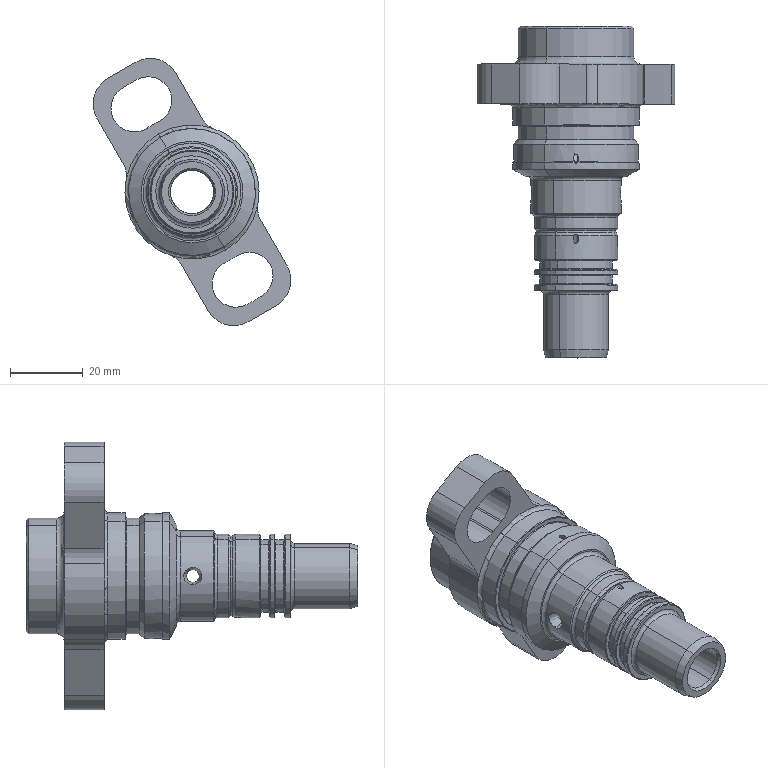Part | SolidWorks | features BaseBody 1 | 1 solid | 175 faces | box 54.543 x 91.5 x 73.761 mm | volume 43286 mm3 | cylinder 76 | torus 37 | cone 37 | plane 25 | commonest cylinder face diameters 1.5 x10 12 x8 13 x8 23 x8 3.5 x4 16 x4